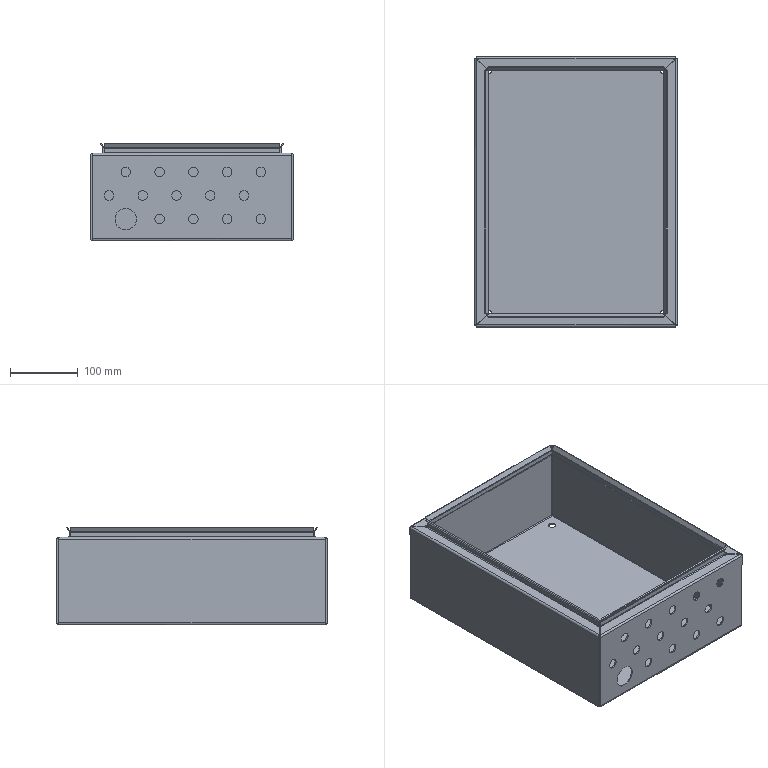Part | SolidWorks | features EdgeFlange 7, 3DProfileFeature 1, Cut 1, FlatPattern 1, HoleWzd 1, ICE 1, SMBaseFlange 1, SheetMetal 1, SketchPattern 1 | 1 solid | 196 faces | box 300 x 400 x 144.964 mm | volume 665331 mm3 | plane 110 | cylinder 70 | spline 16 | commonest cylinder face diameters 14 x28 2 x13 6 x13 11 x8 1.473 x3 5.473 x3